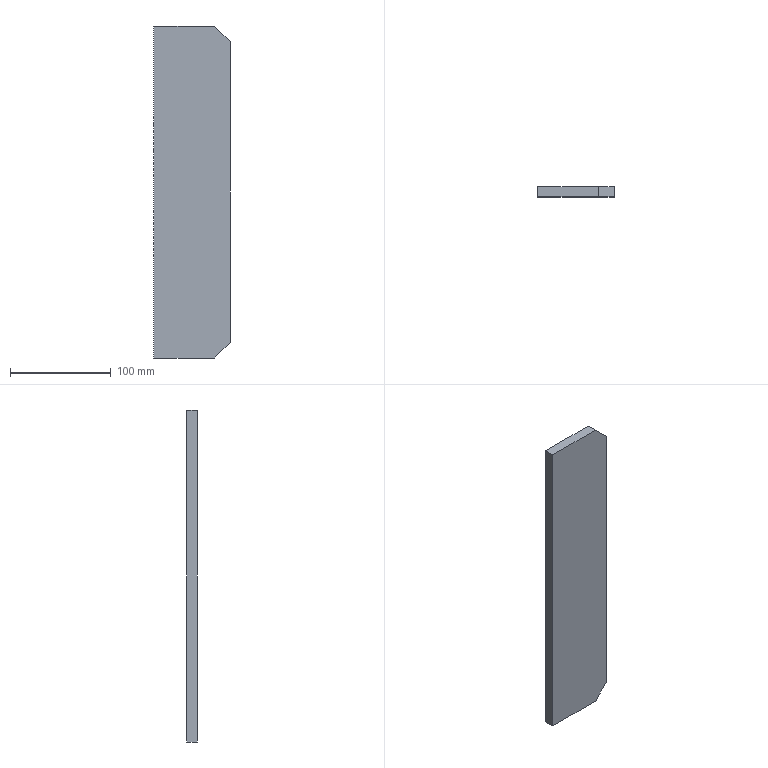Part | SolidWorks | features Extrusion 1 | 1 solid | 8 faces | box 76.2 x 10 x 330.2 mm | volume 249132 mm3 | plane 8
STEP:
#1=CARTESIAN_POINT('',(-40.894,-5.,-140.716));
#2=VERTEX_POINT('',#1);
#3=CARTESIAN_POINT('',(-40.894,-5.,189.484));
#4=VERTEX_POINT('',#3);
#5=CARTESIAN_POINT('',(-40.894,-5.,-140.716));
#6=DIRECTION('',(0.,0.,1.));
#7=VECTOR('',#6,1000.);
#8=LINE('',#5,#7);
#9=EDGE_CURVE('',#2,#4,#8,.T.);
#10=ORIENTED_EDGE('',*,*,#9,.T.);
#11=CARTESIAN_POINT('',(-40.894,5.,189.484));
#12=VERTEX_POINT('',#11);
#13=CARTESIAN_POINT('',(-40.894,5.,189.484));
#14=DIRECTION('',(0.,-1.,0.));
#15=VECTOR('',#14,1000.);
#16=LINE('',#13,#15);
#17=EDGE_CURVE('',#12,#4,#16,.T.);
#18=ORIENTED_EDGE('',*,*,#17,.F.);
#19=CARTESIAN_POINT('',(-40.894,5.,-140.716));
#20=VERTEX_POINT('',#19);
#21=CARTESIAN_POINT('',(-40.894,5.,-140.716));
#22=DIRECTION('',(0.,0.,1.));
#23=VECTOR('',#22,1000.);
#24=LINE('',#21,#23);
#25=EDGE_CURVE('',#20,#12,#24,.T.);
#26=ORIENTED_EDGE('',*,*,#25,.F.);
#27=CARTESIAN_POINT('',(-40.894,5.,-140.716));
#28=DIRECTION('',(0.,-1.,0.));
#29=VECTOR('',#28,1000.);
#30=LINE('',#27,#29);
#31=EDGE_CURVE('',#20,#2,#30,.T.);
#32=ORIENTED_EDGE('',*,*,#31,.T.);
#33=EDGE_LOOP('',(#10,#18,#26,#32));
#34=FACE_OUTER_BOUND('',#33,.T.);
#35=CARTESIAN_POINT('',(-40.894,5.,-140.716));
#36=DIRECTION('',(1.,0.,0.));
#37=DIRECTION('',(0.,0.,-1.));
#38=AXIS2_PLACEMENT_3D('',#35,#36,#37);
#39=PLANE('',#38);
#40=ADVANCED_FACE('',(#34),#39,.F.);
#41=CARTESIAN_POINT('',(19.556,-5.,189.484));
#42=VERTEX_POINT('',#41);
#43=CARTESIAN_POINT('',(-40.894,-5.,189.484));
#44=DIRECTION('',(1.,0.,0.));
#45=VECTOR('',#44,1000.);
#46=LINE('',#43,#45);
#47=EDGE_CURVE('',#4,#42,#46,.T.);
#48=ORIENTED_EDGE('',*,*,#47,.T.);
#49=CARTESIAN_POINT('',(19.556,5.,189.484));
#50=VERTEX_POINT('',#49);
#51=CARTESIAN_POINT('',(19.556,5.,189.484));
#52=DIRECTION('',(0.,-1.,0.));
#53=VECTOR('',#52,1000.);
#54=LINE('',#51,#53);
#55=EDGE_CURVE('',#50,#42,#54,.T.);
#56=ORIENTED_EDGE('',*,*,#55,.F.);
#57=CARTESIAN_POINT('',(-40.894,5.,189.484));
#58=DIRECTION('',(1.,0.,0.));
#59=VECTOR('',#58,1000.);
#60=LINE('',#57,#59);
#61=EDGE_CURVE('',#12,#50,#60,.T.);
#62=ORIENTED_EDGE('',*,*,#61,.F.);
#63=ORIENTED_EDGE('',*,*,#17,.T.);
#64=EDGE_LOOP('',(#48,#56,#62,#63));
#65=FACE_OUTER_BOUND('',#64,.T.);
#66=CARTESIAN_POINT('',(-40.894,5.,189.484));
#67=DIRECTION('',(0.,0.,-1.));
#68=DIRECTION('',(-1.,0.,0.));
#69=AXIS2_PLACEMENT_3D('',#66,#67,#68);
#70=PLANE('',#69);
#71=ADVANCED_FACE('',(#65),#70,.F.);
#72=CARTESIAN_POINT('',(35.306,-5.,173.734));
#73=VERTEX_POINT('',#72);
#74=CARTESIAN_POINT('',(35.306,-5.,173.734));
#75=DIRECTION('',(0.7071,0.,-0.7071));
#76=VECTOR('',#75,1000.);
#77=LINE('',#74,#76);
#78=EDGE_CURVE('',#42,#73,#77,.T.);
#79=ORIENTED_EDGE('',*,*,#78,.T.);
#80=CARTESIAN_POINT('',(35.306,5.,173.734));
#81=VERTEX_POINT('',#80);
#82=CARTESIAN_POINT('',(35.306,5.,173.734));
#83=DIRECTION('',(0.,-1.,0.));
#84=VECTOR('',#83,1000.);
#85=LINE('',#82,#84);
#86=EDGE_CURVE('',#81,#73,#85,.T.);
#87=ORIENTED_EDGE('',*,*,#86,.F.);
#88=CARTESIAN_POINT('',(35.306,5.,173.734));
#89=DIRECTION('',(0.7071,0.,-0.7071));
#90=VECTOR('',#89,1000.);
#91=LINE('',#88,#90);
#92=EDGE_CURVE('',#50,#81,#91,.T.);
#93=ORIENTED_EDGE('',*,*,#92,.F.);
#94=ORIENTED_EDGE('',*,*,#55,.T.);
#95=EDGE_LOOP('',(#79,#87,#93,#94));
#96=FACE_OUTER_BOUND('',#95,.T.);
#97=CARTESIAN_POINT('',(35.306,5.,173.734));
#98=DIRECTION('',(-0.7071,0.,-0.7071));
#99=DIRECTION('',(-0.7071,0.,0.7071));
#100=AXIS2_PLACEMENT_3D('',#97,#98,#99);
#101=PLANE('',#100);
#102=ADVANCED_FACE('',(#96),#101,.F.);
#103=CARTESIAN_POINT('',(35.306,-5.,-124.966));
#104=VERTEX_POINT('',#103);
#105=CARTESIAN_POINT('',(35.306,-5.,-124.966));
#106=DIRECTION('',(0.,0.,-1.));
#107=VECTOR('',#106,1000.);
#108=LINE('',#105,#107);
#109=EDGE_CURVE('',#73,#104,#108,.T.);
#110=ORIENTED_EDGE('',*,*,#109,.T.);
#111=CARTESIAN_POINT('',(35.306,5.,-124.966));
#112=VERTEX_POINT('',#111);
#113=CARTESIAN_POINT('',(35.306,5.,-124.966));
#114=DIRECTION('',(0.,-1.,0.));
#115=VECTOR('',#114,1000.);
#116=LINE('',#113,#115);
#117=EDGE_CURVE('',#112,#104,#116,.T.);
#118=ORIENTED_EDGE('',*,*,#117,.F.);
#119=CARTESIAN_POINT('',(35.306,5.,-124.966));
#120=DIRECTION('',(0.,0.,-1.));
#121=VECTOR('',#120,1000.);
#122=LINE('',#119,#121);
#123=EDGE_CURVE('',#81,#112,#122,.T.);
#124=ORIENTED_EDGE('',*,*,#123,.F.);
#125=ORIENTED_EDGE('',*,*,#86,.T.);
#126=EDGE_LOOP('',(#110,#118,#124,#125));
#127=FACE_OUTER_BOUND('',#126,.T.);
#128=CARTESIAN_POINT('',(35.306,5.,-124.966));
#129=DIRECTION('',(-1.,0.,0.));
#130=DIRECTION('',(0.,0.,1.));
#131=AXIS2_PLACEMENT_3D('',#128,#129,#130);
#132=PLANE('',#131);
#133=ADVANCED_FACE('',(#127),#132,.F.);
#134=CARTESIAN_POINT('',(19.556,-5.,-140.716));
#135=VERTEX_POINT('',#134);
#136=CARTESIAN_POINT('',(19.556,-5.,-140.716));
#137=DIRECTION('',(-0.7071,0.,-0.7071));
#138=VECTOR('',#137,1000.);
#139=LINE('',#136,#138);
#140=EDGE_CURVE('',#104,#135,#139,.T.);
#141=ORIENTED_EDGE('',*,*,#140,.T.);
#142=CARTESIAN_POINT('',(19.556,5.,-140.716));
#143=VERTEX_POINT('',#142);
#144=CARTESIAN_POINT('',(19.556,5.,-140.716));
#145=DIRECTION('',(0.,-1.,0.));
#146=VECTOR('',#145,1000.);
#147=LINE('',#144,#146);
#148=EDGE_CURVE('',#143,#135,#147,.T.);
#149=ORIENTED_EDGE('',*,*,#148,.F.);
#150=CARTESIAN_POINT('',(19.556,5.,-140.716));
#151=DIRECTION('',(-0.7071,0.,-0.7071));
#152=VECTOR('',#151,1000.);
#153=LINE('',#150,#152);
#154=EDGE_CURVE('',#112,#143,#153,.T.);
#155=ORIENTED_EDGE('',*,*,#154,.F.);
#156=ORIENTED_EDGE('',*,*,#117,.T.);
#157=EDGE_LOOP('',(#141,#149,#155,#156));
#158=FACE_OUTER_BOUND('',#157,.T.);
#159=CARTESIAN_POINT('',(19.556,5.,-140.716));
#160=DIRECTION('',(-0.7071,0.,0.7071));
#161=DIRECTION('',(0.7071,0.,0.7071));
#162=AXIS2_PLACEMENT_3D('',#159,#160,#161);
#163=PLANE('',#162);
#164=ADVANCED_FACE('',(#158),#163,.F.);
#165=CARTESIAN_POINT('',(-40.894,-5.,-140.716));
#166=DIRECTION('',(-1.,0.,0.));
#167=VECTOR('',#166,1000.);
#168=LINE('',#165,#167);
#169=EDGE_CURVE('',#135,#2,#168,.T.);
#170=ORIENTED_EDGE('',*,*,#169,.T.);
#171=ORIENTED_EDGE('',*,*,#31,.F.);
#172=CARTESIAN_POINT('',(-40.894,5.,-140.716));
#173=DIRECTION('',(-1.,0.,0.));
#174=VECTOR('',#173,1000.);
#175=LINE('',#172,#174);
#176=EDGE_CURVE('',#143,#20,#175,.T.);
#177=ORIENTED_EDGE('',*,*,#176,.F.);
#178=ORIENTED_EDGE('',*,*,#148,.T.);
#179=EDGE_LOOP('',(#170,#171,#177,#178));
#180=FACE_OUTER_BOUND('',#179,.T.);
#181=CARTESIAN_POINT('',(-40.894,5.,-140.716));
#182=DIRECTION('',(0.,0.,1.));
#183=DIRECTION('',(1.,0.,0.));
#184=AXIS2_PLACEMENT_3D('',#181,#182,#183);
#185=PLANE('',#184);
#186=ADVANCED_FACE('',(#180),#185,.F.);
#187=ORIENTED_EDGE('',*,*,#25,.T.);
#188=ORIENTED_EDGE('',*,*,#61,.T.);
#189=ORIENTED_EDGE('',*,*,#92,.T.);
#190=ORIENTED_EDGE('',*,*,#123,.T.);
#191=ORIENTED_EDGE('',*,*,#154,.T.);
#192=ORIENTED_EDGE('',*,*,#176,.T.);
#193=EDGE_LOOP('',(#187,#188,#189,#190,#191,#192));
#194=FACE_OUTER_BOUND('',#193,.T.);
#195=CARTESIAN_POINT('',(-40.894,5.,189.484));
#196=DIRECTION('',(0.,1.,0.));
#197=DIRECTION('',(0.,0.,1.));
#198=AXIS2_PLACEMENT_3D('',#195,#196,#197);
#199=PLANE('',#198);
#200=ADVANCED_FACE('',(#194),#199,.T.);
#201=ORIENTED_EDGE('',*,*,#9,.F.);
#202=ORIENTED_EDGE('',*,*,#169,.F.);
#203=ORIENTED_EDGE('',*,*,#140,.F.);
#204=ORIENTED_EDGE('',*,*,#109,.F.);
#205=ORIENTED_EDGE('',*,*,#78,.F.);
#206=ORIENTED_EDGE('',*,*,#47,.F.);
#207=EDGE_LOOP('',(#201,#202,#203,#204,#205,#206));
#208=FACE_OUTER_BOUND('',#207,.T.);
#209=CARTESIAN_POINT('',(-40.894,-5.,189.484));
#210=DIRECTION('',(0.,1.,0.));
#211=DIRECTION('',(0.,0.,1.));
#212=AXIS2_PLACEMENT_3D('',#209,#210,#211);
#213=PLANE('',#212);
#214=ADVANCED_FACE('',(#208),#213,.F.);
#215=CLOSED_SHELL('',(#40,#71,#102,#133,#164,#186,#200,#214));
#216=MANIFOLD_SOLID_BREP('',#215);
#217=CARTESIAN_POINT('',(0.,0.,0.));
#218=DIRECTION('',(0.,0.,1.));
#219=DIRECTION('',(1.,0.,0.));
#220=AXIS2_PLACEMENT_3D('',#217,#218,#219);
#221=(LENGTH_UNIT()NAMED_UNIT(*)SI_UNIT(.MILLI.,.METRE.));
#222=UNCERTAINTY_MEASURE_WITH_UNIT(LENGTH_MEASURE(0.00001),#221,'','');
#223=(NAMED_UNIT(*)PLANE_ANGLE_UNIT()SI_UNIT($,.RADIAN.));
#224=(NAMED_UNIT(*)SI_UNIT($,.STERADIAN.)SOLID_ANGLE_UNIT());
#225=(GEOMETRIC_REPRESENTATION_CONTEXT(3)GLOBAL_UNCERTAINTY_ASSIGNED_CONTEXT((#222))GLOBAL_UNIT_ASSIGNED_CONTEXT((#221,#223,#224))REPRESENTATION_CONTEXT('',''));
#226=ADVANCED_BREP_SHAPE_REPRESENTATION('',(#216,#220),#225);